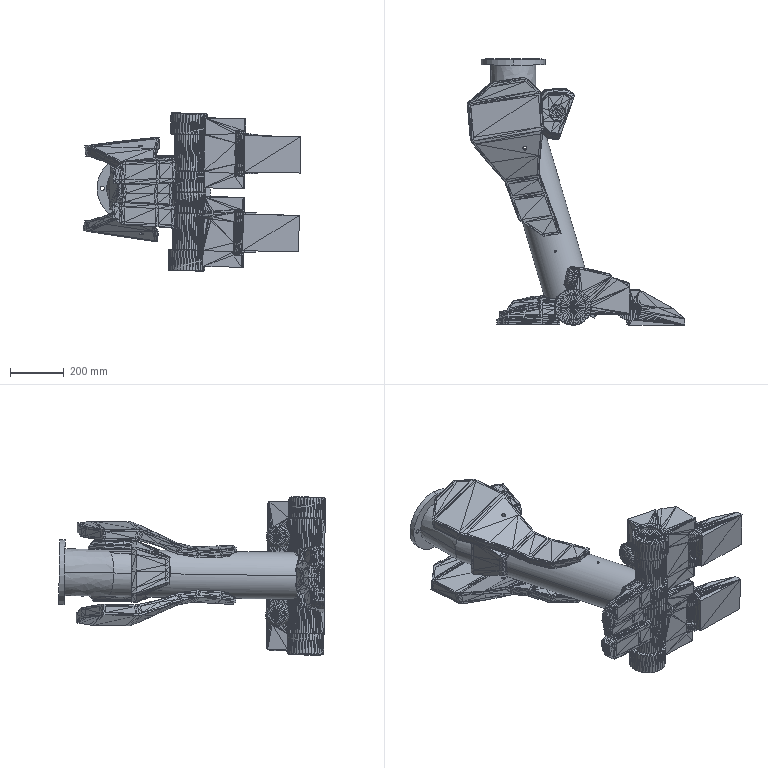Part | SolidWorks | features MirrorStock 1 | 1 solid | 7933 faces | volume 59999692 mm3 | plane 7904 | cylinder 27 | spline 2 | commonest cylinder face diameters 16 x8 8 x6 14.5 x6 300 x3 174.532 x2 240 x2